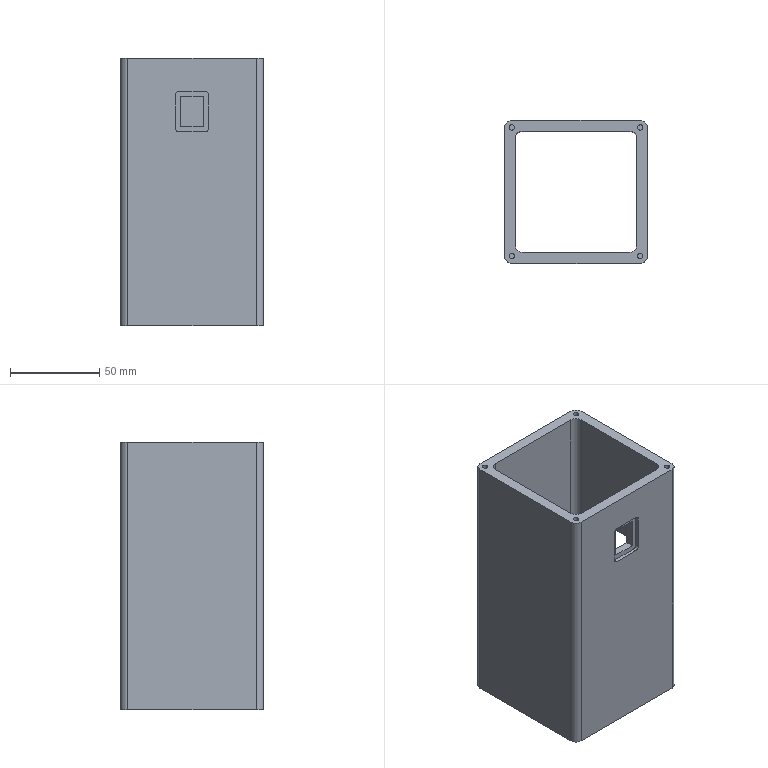Part | SolidWorks | features ICE 7, Fillet 3, Extrusion 1, MirrorPattern 1 | 1 solid | 81 faces | box 80 x 80 x 150 mm | volume 261015 mm3 | plane 45 | cylinder 36 | commonest cylinder face diameters 3 x12 4 x12 8 x7 3.001 x4 8.042 x1